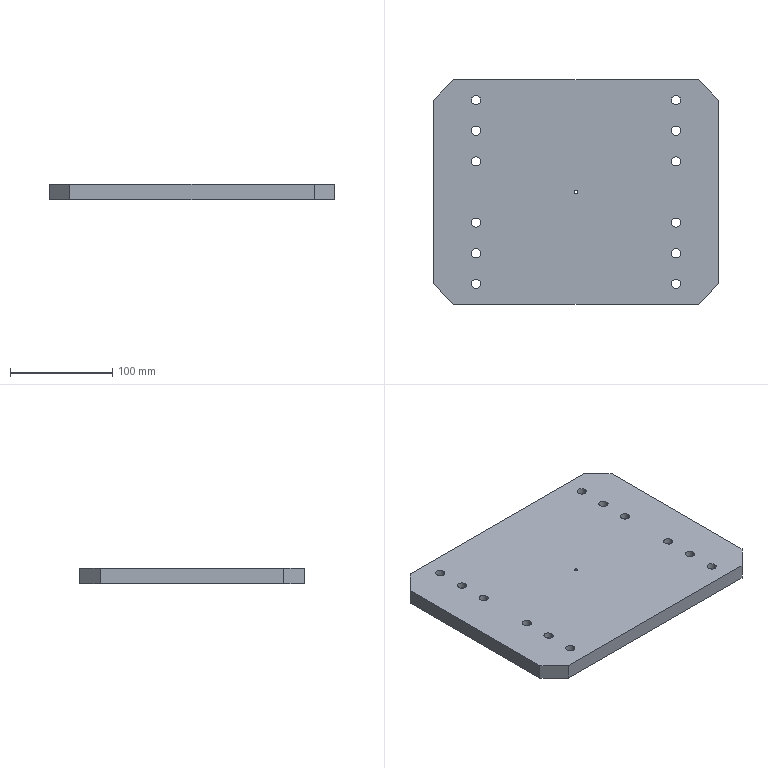Part | STEP file | ASND-0110-Body 1-2 | 1 solid | 72 faces | box 280 x 220 x 15 mm | volume 890688 mm3 | cylinder 50 | plane 22 | commonest cylinder face diameters 9 x24 14 x24 3 x2